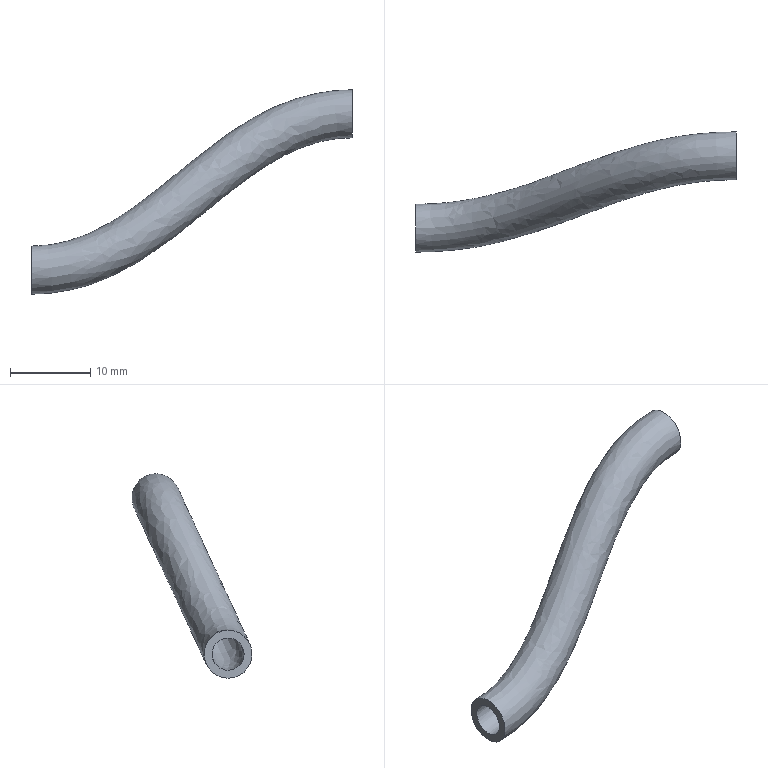Part | NX | features solid 2 | 1 solid | 4 faces | box 40 x 15 x 25.5 mm | volume 731.49 mm3 | plane 2 | spline 2